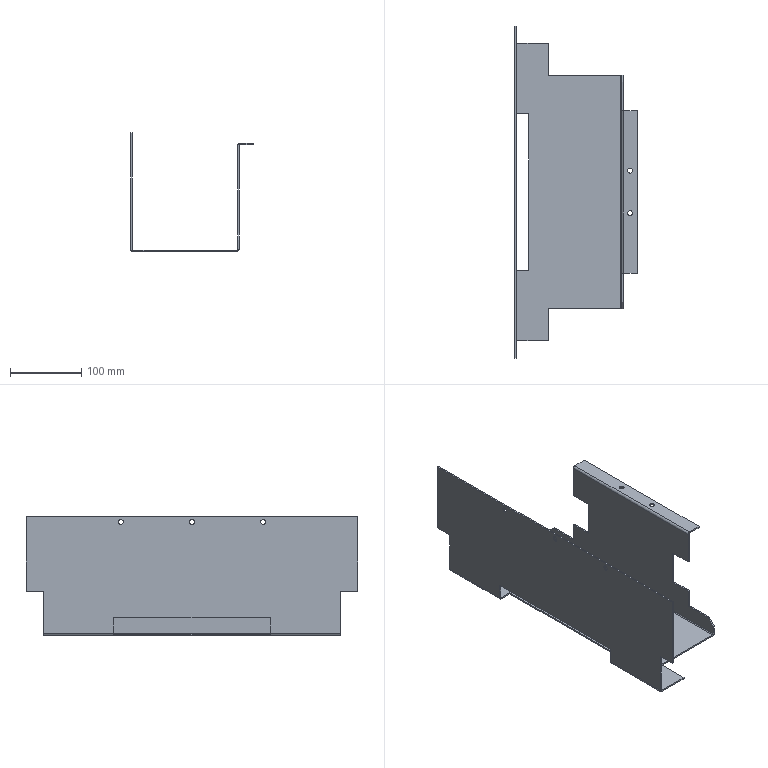Part | SolidWorks | features ICE 6, Cut 2, Fillet 2, Chamfer 1, Extrusion 1 | 1 solid | 56 faces | box 172 x 466 x 167 mm | volume 311713 mm3 | plane 38 | cylinder 18 | commonest cylinder face diameters 7 x10 2 x4 6 x4